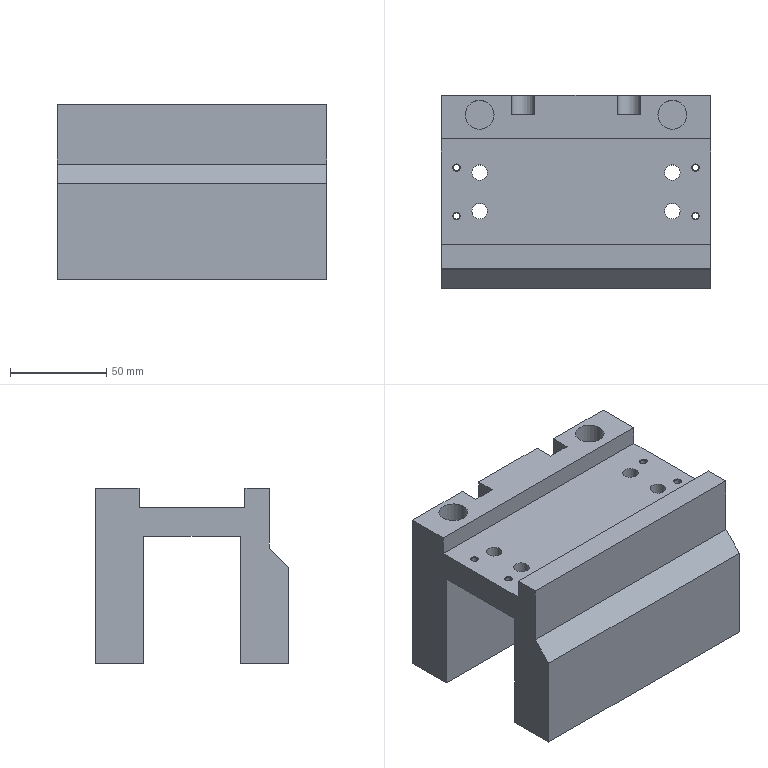Part | STEP file | Tube necking machine_id338_x_t | 1 solid | 44 faces | box 140 x 100 x 91 mm | volume 667813 mm3 | plane 24 | cylinder 12 | cone 8 | commonest cylinder face diameters 3.3 x4 8 x4 12 x2 15 x2